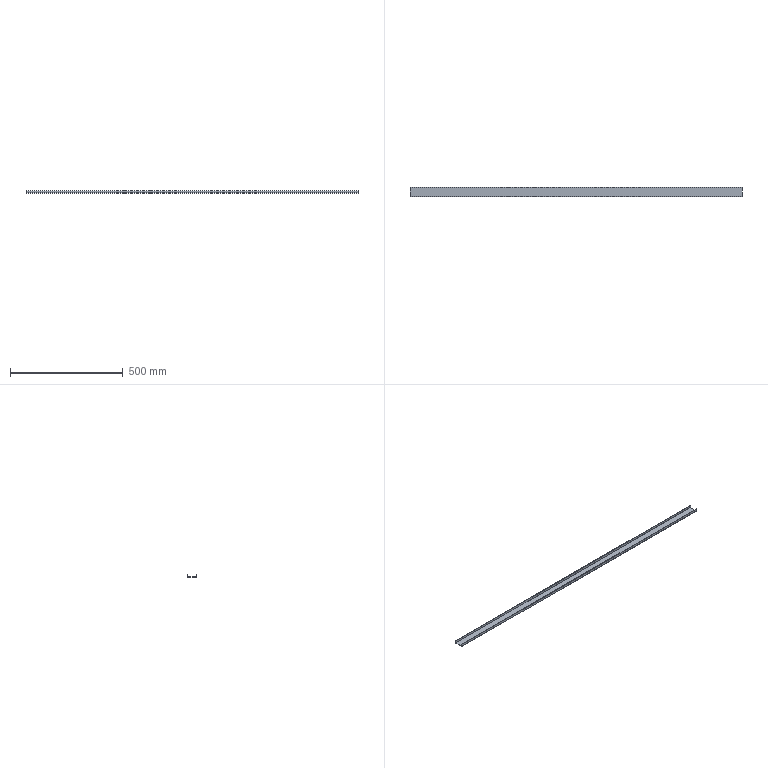Part | SolidWorks | features BaseBody 1, MoveFace 1 | 1 solid | 14 faces | box 1475 x 40 x 12 mm | volume 174214 mm3 | plane 10 | cylinder 4 | commonest cylinder face diameters 0.2 x2 4.2 x2
STEP:
#1=CARTESIAN_POINT('',(-652.5,17.9,-2.));
#2=VERTEX_POINT('',#1);
#3=CARTESIAN_POINT('',(-652.5,-17.9,-2.));
#4=VERTEX_POINT('',#3);
#5=CARTESIAN_POINT('',(-652.5,0.,-2.));
#6=DIRECTION('',(0.,-1.,0.));
#7=VECTOR('',#6,1000.);
#8=LINE('',#5,#7);
#9=EDGE_CURVE('',#2,#4,#8,.T.);
#10=ORIENTED_EDGE('',*,*,#9,.F.);
#11=CARTESIAN_POINT('',(822.5,17.9,-2.));
#12=VERTEX_POINT('',#11);
#13=CARTESIAN_POINT('',(0.,17.9,-2.));
#14=DIRECTION('',(-1.,0.,0.));
#15=VECTOR('',#14,1000.);
#16=LINE('',#13,#15);
#17=EDGE_CURVE('',#12,#2,#16,.T.);
#18=ORIENTED_EDGE('',*,*,#17,.F.);
#19=CARTESIAN_POINT('',(822.5,-17.9,-2.));
#20=VERTEX_POINT('',#19);
#21=CARTESIAN_POINT('',(822.5,0.,-2.));
#22=DIRECTION('',(0.,1.,0.));
#23=VECTOR('',#22,1000.);
#24=LINE('',#21,#23);
#25=EDGE_CURVE('',#20,#12,#24,.T.);
#26=ORIENTED_EDGE('',*,*,#25,.F.);
#27=CARTESIAN_POINT('',(0.,-17.9,-2.));
#28=DIRECTION('',(1.,0.,0.));
#29=VECTOR('',#28,1000.);
#30=LINE('',#27,#29);
#31=EDGE_CURVE('',#4,#20,#30,.T.);
#32=ORIENTED_EDGE('',*,*,#31,.F.);
#33=EDGE_LOOP('',(#10,#18,#26,#32));
#34=FACE_OUTER_BOUND('',#33,.T.);
#35=CARTESIAN_POINT('',(0.,0.,-2.));
#36=DIRECTION('',(0.,0.,1.));
#37=DIRECTION('',(1.,0.,0.));
#38=AXIS2_PLACEMENT_3D('',#35,#36,#37);
#39=PLANE('',#38);
#40=ADVANCED_FACE('',(#34),#39,.F.);
#41=CARTESIAN_POINT('',(822.5,-20.,0.1));
#42=VERTEX_POINT('',#41);
#43=CARTESIAN_POINT('',(-652.5,-20.,0.1));
#44=VERTEX_POINT('',#43);
#45=CARTESIAN_POINT('',(822.5,-20.,0.1));
#46=DIRECTION('',(-1.,0.,0.));
#47=VECTOR('',#46,1000.);
#48=LINE('',#45,#47);
#49=EDGE_CURVE('',#42,#44,#48,.T.);
#50=ORIENTED_EDGE('',*,*,#49,.T.);
#51=CARTESIAN_POINT('',(-652.5,-17.9,0.1));
#52=DIRECTION('',(1.,0.,0.));
#53=DIRECTION('',(0.,0.,-1.));
#54=AXIS2_PLACEMENT_3D('',#51,#52,#53);
#55=CIRCLE('',#54,2.1);
#56=EDGE_CURVE('',#44,#4,#55,.T.);
#57=ORIENTED_EDGE('',*,*,#56,.T.);
#58=ORIENTED_EDGE('',*,*,#31,.T.);
#59=CARTESIAN_POINT('',(822.5,-17.9,0.1));
#60=DIRECTION('',(-1.,0.,0.));
#61=DIRECTION('',(0.,0.,-1.));
#62=AXIS2_PLACEMENT_3D('',#59,#60,#61);
#63=CIRCLE('',#62,2.1);
#64=EDGE_CURVE('',#20,#42,#63,.T.);
#65=ORIENTED_EDGE('',*,*,#64,.T.);
#66=EDGE_LOOP('',(#50,#57,#58,#65));
#67=FACE_OUTER_BOUND('',#66,.T.);
#68=CARTESIAN_POINT('',(822.5,-17.9,0.1));
#69=DIRECTION('',(1.,0.,0.));
#70=DIRECTION('',(0.,0.,-1.));
#71=AXIS2_PLACEMENT_3D('',#68,#69,#70);
#72=CYLINDRICAL_SURFACE('',#71,2.1);
#73=ADVANCED_FACE('',(#67),#72,.T.);
#74=CARTESIAN_POINT('',(-652.5,-17.9,0.));
#75=VERTEX_POINT('',#74);
#76=CARTESIAN_POINT('',(-652.5,17.9,0.));
#77=VERTEX_POINT('',#76);
#78=CARTESIAN_POINT('',(-652.5,20.,0.));
#79=DIRECTION('',(0.,1.,0.));
#80=VECTOR('',#79,1000.);
#81=LINE('',#78,#80);
#82=EDGE_CURVE('',#75,#77,#81,.T.);
#83=ORIENTED_EDGE('',*,*,#82,.T.);
#84=CARTESIAN_POINT('',(-652.5,18.,0.1));
#85=VERTEX_POINT('',#84);
#86=CARTESIAN_POINT('',(-652.5,17.9,0.1));
#87=DIRECTION('',(1.,0.,0.));
#88=DIRECTION('',(0.,0.,1.));
#89=AXIS2_PLACEMENT_3D('',#86,#87,#88);
#90=CIRCLE('',#89,0.1);
#91=EDGE_CURVE('',#77,#85,#90,.T.);
#92=ORIENTED_EDGE('',*,*,#91,.T.);
#93=CARTESIAN_POINT('',(-652.5,18.,10.));
#94=VERTEX_POINT('',#93);
#95=CARTESIAN_POINT('',(-652.5,18.,10.));
#96=DIRECTION('',(0.,0.,-1.));
#97=VECTOR('',#96,1000.);
#98=LINE('',#95,#97);
#99=EDGE_CURVE('',#94,#85,#98,.T.);
#100=ORIENTED_EDGE('',*,*,#99,.F.);
#101=CARTESIAN_POINT('',(-652.5,20.,10.));
#102=VERTEX_POINT('',#101);
#103=CARTESIAN_POINT('',(-652.5,20.,10.));
#104=DIRECTION('',(0.,-1.,0.));
#105=VECTOR('',#104,1000.);
#106=LINE('',#103,#105);
#107=EDGE_CURVE('',#102,#94,#106,.T.);
#108=ORIENTED_EDGE('',*,*,#107,.F.);
#109=CARTESIAN_POINT('',(-652.5,20.,0.1));
#110=VERTEX_POINT('',#109);
#111=CARTESIAN_POINT('',(-652.5,20.,0.));
#112=DIRECTION('',(0.,0.,-1.));
#113=VECTOR('',#112,1000.);
#114=LINE('',#111,#113);
#115=EDGE_CURVE('',#102,#110,#114,.T.);
#116=ORIENTED_EDGE('',*,*,#115,.T.);
#117=CARTESIAN_POINT('',(-652.5,17.9,0.1));
#118=DIRECTION('',(1.,0.,0.));
#119=DIRECTION('',(0.,0.,1.));
#120=AXIS2_PLACEMENT_3D('',#117,#118,#119);
#121=CIRCLE('',#120,2.1);
#122=EDGE_CURVE('',#2,#110,#121,.T.);
#123=ORIENTED_EDGE('',*,*,#122,.F.);
#124=ORIENTED_EDGE('',*,*,#9,.T.);
#125=ORIENTED_EDGE('',*,*,#56,.F.);
#126=CARTESIAN_POINT('',(-652.5,-20.,10.));
#127=VERTEX_POINT('',#126);
#128=CARTESIAN_POINT('',(-652.5,-20.,0.));
#129=DIRECTION('',(0.,0.,1.));
#130=VECTOR('',#129,1000.);
#131=LINE('',#128,#130);
#132=EDGE_CURVE('',#44,#127,#131,.T.);
#133=ORIENTED_EDGE('',*,*,#132,.T.);
#134=CARTESIAN_POINT('',(-652.5,-18.,10.));
#135=VERTEX_POINT('',#134);
#136=CARTESIAN_POINT('',(-652.5,-20.,10.));
#137=DIRECTION('',(0.,-1.,0.));
#138=VECTOR('',#137,1000.);
#139=LINE('',#136,#138);
#140=EDGE_CURVE('',#135,#127,#139,.T.);
#141=ORIENTED_EDGE('',*,*,#140,.F.);
#142=CARTESIAN_POINT('',(-652.5,-18.,0.1));
#143=VERTEX_POINT('',#142);
#144=CARTESIAN_POINT('',(-652.5,-18.,0.));
#145=DIRECTION('',(0.,0.,1.));
#146=VECTOR('',#145,1000.);
#147=LINE('',#144,#146);
#148=EDGE_CURVE('',#143,#135,#147,.T.);
#149=ORIENTED_EDGE('',*,*,#148,.F.);
#150=CARTESIAN_POINT('',(-652.5,-17.9,0.1));
#151=DIRECTION('',(1.,0.,0.));
#152=DIRECTION('',(0.,0.,-1.));
#153=AXIS2_PLACEMENT_3D('',#150,#151,#152);
#154=CIRCLE('',#153,0.1);
#155=EDGE_CURVE('',#143,#75,#154,.T.);
#156=ORIENTED_EDGE('',*,*,#155,.T.);
#157=EDGE_LOOP('',(#83,#92,#100,#108,#116,#123,#124,#125,#133,#141,#149,#156));
#158=FACE_OUTER_BOUND('',#157,.T.);
#159=CARTESIAN_POINT('',(-652.5,20.,-2.));
#160=DIRECTION('',(-1.,0.,0.));
#161=DIRECTION('',(0.,0.,1.));
#162=AXIS2_PLACEMENT_3D('',#159,#160,#161);
#163=PLANE('',#162);
#164=ADVANCED_FACE('',(#158),#163,.T.);
#165=CARTESIAN_POINT('',(822.5,20.,0.1));
#166=VERTEX_POINT('',#165);
#167=CARTESIAN_POINT('',(-822.5,20.,0.1));
#168=DIRECTION('',(1.,0.,0.));
#169=VECTOR('',#168,1000.);
#170=LINE('',#167,#169);
#171=EDGE_CURVE('',#110,#166,#170,.T.);
#172=ORIENTED_EDGE('',*,*,#171,.T.);
#173=CARTESIAN_POINT('',(822.5,17.9,0.1));
#174=DIRECTION('',(-1.,0.,0.));
#175=DIRECTION('',(0.,0.,1.));
#176=AXIS2_PLACEMENT_3D('',#173,#174,#175);
#177=CIRCLE('',#176,2.1);
#178=EDGE_CURVE('',#166,#12,#177,.T.);
#179=ORIENTED_EDGE('',*,*,#178,.T.);
#180=ORIENTED_EDGE('',*,*,#17,.T.);
#181=ORIENTED_EDGE('',*,*,#122,.T.);
#182=EDGE_LOOP('',(#172,#179,#180,#181));
#183=FACE_OUTER_BOUND('',#182,.T.);
#184=CARTESIAN_POINT('',(-822.5,17.9,0.1));
#185=DIRECTION('',(-1.,0.,0.));
#186=DIRECTION('',(0.,0.,1.));
#187=AXIS2_PLACEMENT_3D('',#184,#185,#186);
#188=CYLINDRICAL_SURFACE('',#187,2.1);
#189=ADVANCED_FACE('',(#183),#188,.T.);
#190=ORIENTED_EDGE('',*,*,#25,.T.);
#191=ORIENTED_EDGE('',*,*,#178,.F.);
#192=CARTESIAN_POINT('',(822.5,20.,10.));
#193=VERTEX_POINT('',#192);
#194=CARTESIAN_POINT('',(822.5,20.,0.));
#195=DIRECTION('',(0.,0.,1.));
#196=VECTOR('',#195,1000.);
#197=LINE('',#194,#196);
#198=EDGE_CURVE('',#166,#193,#197,.T.);
#199=ORIENTED_EDGE('',*,*,#198,.T.);
#200=CARTESIAN_POINT('',(822.5,18.,10.));
#201=VERTEX_POINT('',#200);
#202=CARTESIAN_POINT('',(822.5,20.,10.));
#203=DIRECTION('',(0.,1.,0.));
#204=VECTOR('',#203,1000.);
#205=LINE('',#202,#204);
#206=EDGE_CURVE('',#201,#193,#205,.T.);
#207=ORIENTED_EDGE('',*,*,#206,.F.);
#208=CARTESIAN_POINT('',(822.5,18.,0.1));
#209=VERTEX_POINT('',#208);
#210=CARTESIAN_POINT('',(822.5,18.,0.));
#211=DIRECTION('',(0.,0.,1.));
#212=VECTOR('',#211,1000.);
#213=LINE('',#210,#212);
#214=EDGE_CURVE('',#209,#201,#213,.T.);
#215=ORIENTED_EDGE('',*,*,#214,.F.);
#216=CARTESIAN_POINT('',(822.5,17.9,0.));
#217=VERTEX_POINT('',#216);
#218=CARTESIAN_POINT('',(822.5,17.9,0.1));
#219=DIRECTION('',(-1.,0.,0.));
#220=DIRECTION('',(0.,0.,1.));
#221=AXIS2_PLACEMENT_3D('',#218,#219,#220);
#222=CIRCLE('',#221,0.1);
#223=EDGE_CURVE('',#209,#217,#222,.T.);
#224=ORIENTED_EDGE('',*,*,#223,.T.);
#225=CARTESIAN_POINT('',(822.5,-17.9,0.));
#226=VERTEX_POINT('',#225);
#227=CARTESIAN_POINT('',(822.5,20.,0.));
#228=DIRECTION('',(0.,-1.,0.));
#229=VECTOR('',#228,1000.);
#230=LINE('',#227,#229);
#231=EDGE_CURVE('',#217,#226,#230,.T.);
#232=ORIENTED_EDGE('',*,*,#231,.T.);
#233=CARTESIAN_POINT('',(822.5,-18.,0.1));
#234=VERTEX_POINT('',#233);
#235=CARTESIAN_POINT('',(822.5,-17.9,0.1));
#236=DIRECTION('',(-1.,0.,0.));
#237=DIRECTION('',(0.,0.,-1.));
#238=AXIS2_PLACEMENT_3D('',#235,#236,#237);
#239=CIRCLE('',#238,0.1);
#240=EDGE_CURVE('',#226,#234,#239,.T.);
#241=ORIENTED_EDGE('',*,*,#240,.T.);
#242=CARTESIAN_POINT('',(822.5,-18.,10.));
#243=VERTEX_POINT('',#242);
#244=CARTESIAN_POINT('',(822.5,-18.,10.));
#245=DIRECTION('',(0.,0.,-1.));
#246=VECTOR('',#245,1000.);
#247=LINE('',#244,#246);
#248=EDGE_CURVE('',#243,#234,#247,.T.);
#249=ORIENTED_EDGE('',*,*,#248,.F.);
#250=CARTESIAN_POINT('',(822.5,-20.,10.));
#251=VERTEX_POINT('',#250);
#252=CARTESIAN_POINT('',(822.5,-20.,10.));
#253=DIRECTION('',(0.,1.,0.));
#254=VECTOR('',#253,1000.);
#255=LINE('',#252,#254);
#256=EDGE_CURVE('',#251,#243,#255,.T.);
#257=ORIENTED_EDGE('',*,*,#256,.F.);
#258=CARTESIAN_POINT('',(822.5,-20.,0.));
#259=DIRECTION('',(0.,0.,-1.));
#260=VECTOR('',#259,1000.);
#261=LINE('',#258,#260);
#262=EDGE_CURVE('',#251,#42,#261,.T.);
#263=ORIENTED_EDGE('',*,*,#262,.T.);
#264=ORIENTED_EDGE('',*,*,#64,.F.);
#265=EDGE_LOOP('',(#190,#191,#199,#207,#215,#224,#232,#241,#249,#257,#263,#264));
#266=FACE_OUTER_BOUND('',#265,.T.);
#267=CARTESIAN_POINT('',(822.5,20.,-2.));
#268=DIRECTION('',(1.,0.,0.));
#269=DIRECTION('',(0.,0.,-1.));
#270=AXIS2_PLACEMENT_3D('',#267,#268,#269);
#271=PLANE('',#270);
#272=ADVANCED_FACE('',(#266),#271,.T.);
#273=ORIENTED_EDGE('',*,*,#262,.F.);
#274=CARTESIAN_POINT('',(0.,-20.,10.));
#275=DIRECTION('',(1.,0.,0.));
#276=VECTOR('',#275,1000.);
#277=LINE('',#274,#276);
#278=EDGE_CURVE('',#127,#251,#277,.T.);
#279=ORIENTED_EDGE('',*,*,#278,.F.);
#280=ORIENTED_EDGE('',*,*,#132,.F.);
#281=ORIENTED_EDGE('',*,*,#49,.F.);
#282=EDGE_LOOP('',(#273,#279,#280,#281));
#283=FACE_OUTER_BOUND('',#282,.T.);
#284=CARTESIAN_POINT('',(0.,-20.,0.));
#285=DIRECTION('',(0.,1.,0.));
#286=DIRECTION('',(0.,0.,1.));
#287=AXIS2_PLACEMENT_3D('',#284,#285,#286);
#288=PLANE('',#287);
#289=ADVANCED_FACE('',(#283),#288,.F.);
#290=ORIENTED_EDGE('',*,*,#231,.F.);
#291=CARTESIAN_POINT('',(0.,17.9,0.));
#292=DIRECTION('',(-1.,0.,0.));
#293=VECTOR('',#292,1000.);
#294=LINE('',#291,#293);
#295=EDGE_CURVE('',#217,#77,#294,.T.);
#296=ORIENTED_EDGE('',*,*,#295,.T.);
#297=ORIENTED_EDGE('',*,*,#82,.F.);
#298=CARTESIAN_POINT('',(0.,-17.9,0.));
#299=DIRECTION('',(1.,0.,0.));
#300=VECTOR('',#299,1000.);
#301=LINE('',#298,#300);
#302=EDGE_CURVE('',#75,#226,#301,.T.);
#303=ORIENTED_EDGE('',*,*,#302,.T.);
#304=EDGE_LOOP('',(#290,#296,#297,#303));
#305=FACE_OUTER_BOUND('',#304,.T.);
#306=CARTESIAN_POINT('',(0.,0.,0.));
#307=DIRECTION('',(0.,0.,1.));
#308=DIRECTION('',(1.,0.,0.));
#309=AXIS2_PLACEMENT_3D('',#306,#307,#308);
#310=PLANE('',#309);
#311=ADVANCED_FACE('',(#305),#310,.T.);
#312=ORIENTED_EDGE('',*,*,#115,.F.);
#313=CARTESIAN_POINT('',(0.,20.,10.));
#314=DIRECTION('',(-1.,0.,0.));
#315=VECTOR('',#314,1000.);
#316=LINE('',#313,#315);
#317=EDGE_CURVE('',#193,#102,#316,.T.);
#318=ORIENTED_EDGE('',*,*,#317,.F.);
#319=ORIENTED_EDGE('',*,*,#198,.F.);
#320=ORIENTED_EDGE('',*,*,#171,.F.);
#321=EDGE_LOOP('',(#312,#318,#319,#320));
#322=FACE_OUTER_BOUND('',#321,.T.);
#323=CARTESIAN_POINT('',(0.,20.,0.));
#324=DIRECTION('',(0.,-1.,0.));
#325=DIRECTION('',(0.,0.,-1.));
#326=AXIS2_PLACEMENT_3D('',#323,#324,#325);
#327=PLANE('',#326);
#328=ADVANCED_FACE('',(#322),#327,.F.);
#329=ORIENTED_EDGE('',*,*,#140,.T.);
#330=ORIENTED_EDGE('',*,*,#278,.T.);
#331=ORIENTED_EDGE('',*,*,#256,.T.);
#332=CARTESIAN_POINT('',(-822.5,-18.,10.));
#333=DIRECTION('',(1.,0.,0.));
#334=VECTOR('',#333,1000.);
#335=LINE('',#332,#334);
#336=EDGE_CURVE('',#135,#243,#335,.T.);
#337=ORIENTED_EDGE('',*,*,#336,.F.);
#338=EDGE_LOOP('',(#329,#330,#331,#337));
#339=FACE_OUTER_BOUND('',#338,.T.);
#340=CARTESIAN_POINT('',(-822.5,-20.,10.));
#341=DIRECTION('',(0.,0.,-1.));
#342=DIRECTION('',(0.,1.,0.));
#343=AXIS2_PLACEMENT_3D('',#340,#341,#342);
#344=PLANE('',#343);
#345=ADVANCED_FACE('',(#339),#344,.F.);
#346=ORIENTED_EDGE('',*,*,#223,.F.);
#347=CARTESIAN_POINT('',(-822.5,18.,0.1));
#348=DIRECTION('',(1.,0.,0.));
#349=VECTOR('',#348,1000.);
#350=LINE('',#347,#349);
#351=EDGE_CURVE('',#85,#209,#350,.T.);
#352=ORIENTED_EDGE('',*,*,#351,.F.);
#353=ORIENTED_EDGE('',*,*,#91,.F.);
#354=ORIENTED_EDGE('',*,*,#295,.F.);
#355=EDGE_LOOP('',(#346,#352,#353,#354));
#356=FACE_OUTER_BOUND('',#355,.T.);
#357=CARTESIAN_POINT('',(-822.5,17.9,0.1));
#358=DIRECTION('',(-1.,0.,0.));
#359=DIRECTION('',(0.,0.,1.));
#360=AXIS2_PLACEMENT_3D('',#357,#358,#359);
#361=CYLINDRICAL_SURFACE('',#360,0.1);
#362=ADVANCED_FACE('',(#356),#361,.F.);
#363=ORIENTED_EDGE('',*,*,#155,.F.);
#364=CARTESIAN_POINT('',(822.5,-18.,0.1));
#365=DIRECTION('',(-1.,0.,0.));
#366=VECTOR('',#365,1000.);
#367=LINE('',#364,#366);
#368=EDGE_CURVE('',#234,#143,#367,.T.);
#369=ORIENTED_EDGE('',*,*,#368,.F.);
#370=ORIENTED_EDGE('',*,*,#240,.F.);
#371=ORIENTED_EDGE('',*,*,#302,.F.);
#372=EDGE_LOOP('',(#363,#369,#370,#371));
#373=FACE_OUTER_BOUND('',#372,.T.);
#374=CARTESIAN_POINT('',(822.5,-17.9,0.1));
#375=DIRECTION('',(1.,0.,0.));
#376=DIRECTION('',(0.,0.,-1.));
#377=AXIS2_PLACEMENT_3D('',#374,#375,#376);
#378=CYLINDRICAL_SURFACE('',#377,0.1);
#379=ADVANCED_FACE('',(#373),#378,.F.);
#380=ORIENTED_EDGE('',*,*,#206,.T.);
#381=ORIENTED_EDGE('',*,*,#317,.T.);
#382=ORIENTED_EDGE('',*,*,#107,.T.);
#383=CARTESIAN_POINT('',(822.5,18.,10.));
#384=DIRECTION('',(-1.,0.,0.));
#385=VECTOR('',#384,1000.);
#386=LINE('',#383,#385);
#387=EDGE_CURVE('',#201,#94,#386,.T.);
#388=ORIENTED_EDGE('',*,*,#387,.F.);
#389=EDGE_LOOP('',(#380,#381,#382,#388));
#390=FACE_OUTER_BOUND('',#389,.T.);
#391=CARTESIAN_POINT('',(822.5,20.,10.));
#392=DIRECTION('',(0.,0.,-1.));
#393=DIRECTION('',(0.,1.,0.));
#394=AXIS2_PLACEMENT_3D('',#391,#392,#393);
#395=PLANE('',#394);
#396=ADVANCED_FACE('',(#390),#395,.F.);
#397=ORIENTED_EDGE('',*,*,#148,.T.);
#398=ORIENTED_EDGE('',*,*,#336,.T.);
#399=ORIENTED_EDGE('',*,*,#248,.T.);
#400=ORIENTED_EDGE('',*,*,#368,.T.);
#401=EDGE_LOOP('',(#397,#398,#399,#400));
#402=FACE_OUTER_BOUND('',#401,.T.);
#403=CARTESIAN_POINT('',(0.,-18.,0.));
#404=DIRECTION('',(0.,1.,0.));
#405=DIRECTION('',(0.,0.,1.));
#406=AXIS2_PLACEMENT_3D('',#403,#404,#405);
#407=PLANE('',#406);
#408=ADVANCED_FACE('',(#402),#407,.T.);
#409=ORIENTED_EDGE('',*,*,#214,.T.);
#410=ORIENTED_EDGE('',*,*,#387,.T.);
#411=ORIENTED_EDGE('',*,*,#99,.T.);
#412=ORIENTED_EDGE('',*,*,#351,.T.);
#413=EDGE_LOOP('',(#409,#410,#411,#412));
#414=FACE_OUTER_BOUND('',#413,.T.);
#415=CARTESIAN_POINT('',(0.,18.,0.));
#416=DIRECTION('',(0.,-1.,0.));
#417=DIRECTION('',(0.,0.,-1.));
#418=AXIS2_PLACEMENT_3D('',#415,#416,#417);
#419=PLANE('',#418);
#420=ADVANCED_FACE('',(#414),#419,.T.);
#421=CLOSED_SHELL('',(#40,#73,#164,#189,#272,#289,#311,#328,#345,#362,#379,#396,#408,#420));
#422=MANIFOLD_SOLID_BREP('',#421);
#423=CARTESIAN_POINT('',(0.,0.,0.));
#424=DIRECTION('',(0.,0.,1.));
#425=DIRECTION('',(1.,0.,0.));
#426=AXIS2_PLACEMENT_3D('',#423,#424,#425);
#427=(LENGTH_UNIT()NAMED_UNIT(*)SI_UNIT(.MILLI.,.METRE.));
#428=UNCERTAINTY_MEASURE_WITH_UNIT(LENGTH_MEASURE(0.00001),#427,'','');
#429=(NAMED_UNIT(*)PLANE_ANGLE_UNIT()SI_UNIT($,.RADIAN.));
#430=(NAMED_UNIT(*)SI_UNIT($,.STERADIAN.)SOLID_ANGLE_UNIT());
#431=(GEOMETRIC_REPRESENTATION_CONTEXT(3)GLOBAL_UNCERTAINTY_ASSIGNED_CONTEXT((#428))GLOBAL_UNIT_ASSIGNED_CONTEXT((#427,#429,#430))REPRESENTATION_CONTEXT('',''));
#432=ADVANCED_BREP_SHAPE_REPRESENTATION('',(#422,#426),#431);